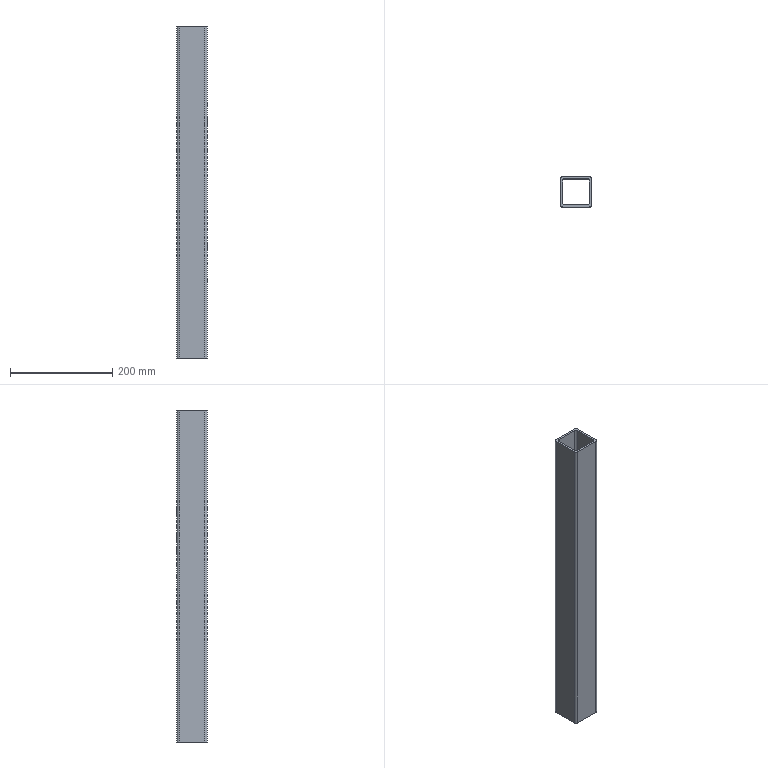Part | STEP file | 1 solid | 62 faces | box 60 x 60 x 650 mm | volume 580718 mm3 | cylinder 52 | plane 10 | commonest cylinder face diameters 5 x40 10 x8 4.2 x4